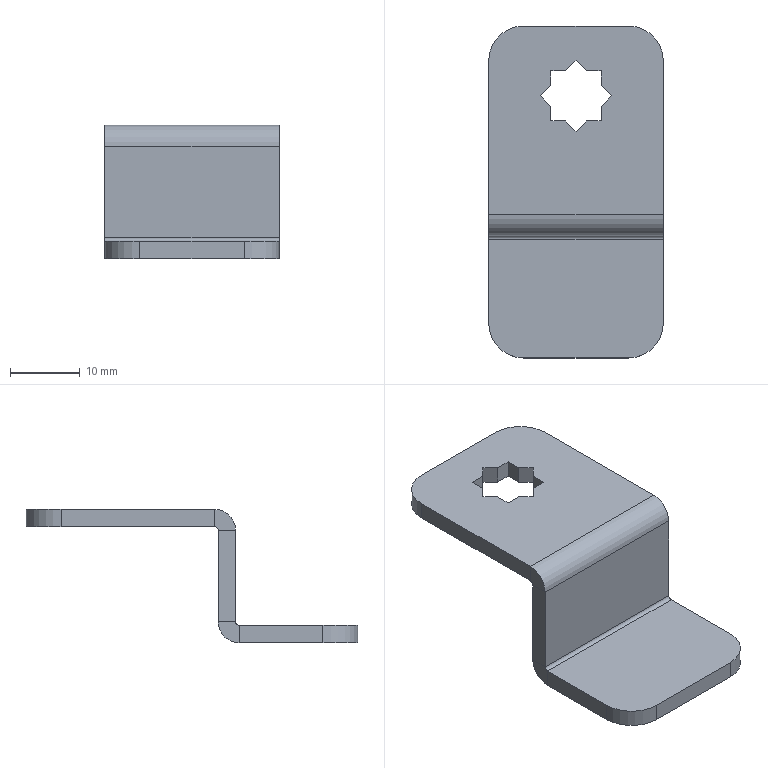Part | SolidWorks | features BaseBody 1 | 1 solid | 42 faces | box 25 x 47.5 x 19.1 mm | volume 3707 mm3 | plane 34 | cylinder 8 | commonest cylinder face diameters 10 x4 1 x2 6 x2
STEP:
#1=CARTESIAN_POINT('',(5.091,5.,0.));
#2=VERTEX_POINT('',#1);
#3=CARTESIAN_POINT('',(3.6,3.509,0.));
#4=VERTEX_POINT('',#3);
#5=CARTESIAN_POINT('',(5.091,5.,0.));
#6=DIRECTION('',(-0.7071,-0.7071,0.));
#7=VECTOR('',#6,1000.);
#8=LINE('',#5,#7);
#9=EDGE_CURVE('',#2,#4,#8,.T.);
#10=ORIENTED_EDGE('',*,*,#9,.F.);
#11=CARTESIAN_POINT('',(5.091,5.,-2.5));
#12=VERTEX_POINT('',#11);
#13=CARTESIAN_POINT('',(5.091,5.,0.));
#14=DIRECTION('',(0.,0.,-1.));
#15=VECTOR('',#14,1000.);
#16=LINE('',#13,#15);
#17=EDGE_CURVE('',#2,#12,#16,.T.);
#18=ORIENTED_EDGE('',*,*,#17,.T.);
#19=CARTESIAN_POINT('',(3.6,3.509,-2.5));
#20=VERTEX_POINT('',#19);
#21=CARTESIAN_POINT('',(5.091,5.,-2.5));
#22=DIRECTION('',(-0.7071,-0.7071,0.));
#23=VECTOR('',#22,1000.);
#24=LINE('',#21,#23);
#25=EDGE_CURVE('',#12,#20,#24,.T.);
#26=ORIENTED_EDGE('',*,*,#25,.T.);
#27=CARTESIAN_POINT('',(3.6,3.509,0.));
#28=DIRECTION('',(0.,0.,-1.));
#29=VECTOR('',#28,1000.);
#30=LINE('',#27,#29);
#31=EDGE_CURVE('',#4,#20,#30,.T.);
#32=ORIENTED_EDGE('',*,*,#31,.F.);
#33=EDGE_LOOP('',(#10,#18,#26,#32));
#34=FACE_OUTER_BOUND('',#33,.T.);
#35=CARTESIAN_POINT('',(5.091,5.,0.));
#36=DIRECTION('',(0.7071,-0.7071,0.));
#37=DIRECTION('',(0.,0.,-1.));
#38=AXIS2_PLACEMENT_3D('',#35,#36,#37);
#39=PLANE('',#38);
#40=ADVANCED_FACE('',(#34),#39,.F.);
#41=CARTESIAN_POINT('',(3.6,6.491,-2.5));
#42=VERTEX_POINT('',#41);
#43=CARTESIAN_POINT('',(0.,10.091,-2.5));
#44=DIRECTION('',(0.7071,-0.7071,0.));
#45=VECTOR('',#44,1000.);
#46=LINE('',#43,#45);
#47=EDGE_CURVE('',#42,#12,#46,.T.);
#48=ORIENTED_EDGE('',*,*,#47,.T.);
#49=ORIENTED_EDGE('',*,*,#17,.F.);
#50=CARTESIAN_POINT('',(3.6,6.491,0.));
#51=VERTEX_POINT('',#50);
#52=CARTESIAN_POINT('',(0.,10.091,0.));
#53=DIRECTION('',(0.7071,-0.7071,0.));
#54=VECTOR('',#53,1000.);
#55=LINE('',#52,#54);
#56=EDGE_CURVE('',#51,#2,#55,.T.);
#57=ORIENTED_EDGE('',*,*,#56,.F.);
#58=CARTESIAN_POINT('',(3.6,6.491,0.));
#59=DIRECTION('',(0.,0.,1.));
#60=VECTOR('',#59,1000.);
#61=LINE('',#58,#60);
#62=EDGE_CURVE('',#42,#51,#61,.T.);
#63=ORIENTED_EDGE('',*,*,#62,.F.);
#64=EDGE_LOOP('',(#48,#49,#57,#63));
#65=FACE_OUTER_BOUND('',#64,.T.);
#66=CARTESIAN_POINT('',(0.,10.091,0.));
#67=DIRECTION('',(0.7071,0.7071,0.));
#68=DIRECTION('',(0.,0.,-1.));
#69=AXIS2_PLACEMENT_3D('',#66,#67,#68);
#70=PLANE('',#69);
#71=ADVANCED_FACE('',(#65),#70,.F.);
#72=CARTESIAN_POINT('',(0.,10.091,0.));
#73=VERTEX_POINT('',#72);
#74=CARTESIAN_POINT('',(1.491,8.6,0.));
#75=VERTEX_POINT('',#74);
#76=CARTESIAN_POINT('',(0.,10.091,0.));
#77=DIRECTION('',(0.7071,-0.7071,0.));
#78=VECTOR('',#77,1000.);
#79=LINE('',#76,#78);
#80=EDGE_CURVE('',#73,#75,#79,.T.);
#81=ORIENTED_EDGE('',*,*,#80,.F.);
#82=CARTESIAN_POINT('',(0.,10.091,-2.5));
#83=VERTEX_POINT('',#82);
#84=CARTESIAN_POINT('',(0.,10.091,0.));
#85=DIRECTION('',(0.,0.,-1.));
#86=VECTOR('',#85,1000.);
#87=LINE('',#84,#86);
#88=EDGE_CURVE('',#73,#83,#87,.T.);
#89=ORIENTED_EDGE('',*,*,#88,.T.);
#90=CARTESIAN_POINT('',(1.491,8.6,-2.5));
#91=VERTEX_POINT('',#90);
#92=CARTESIAN_POINT('',(0.,10.091,-2.5));
#93=DIRECTION('',(0.7071,-0.7071,0.));
#94=VECTOR('',#93,1000.);
#95=LINE('',#92,#94);
#96=EDGE_CURVE('',#83,#91,#95,.T.);
#97=ORIENTED_EDGE('',*,*,#96,.T.);
#98=CARTESIAN_POINT('',(1.491,8.6,0.));
#99=DIRECTION('',(0.,0.,-1.));
#100=VECTOR('',#99,1000.);
#101=LINE('',#98,#100);
#102=EDGE_CURVE('',#75,#91,#101,.T.);
#103=ORIENTED_EDGE('',*,*,#102,.F.);
#104=EDGE_LOOP('',(#81,#89,#97,#103));
#105=FACE_OUTER_BOUND('',#104,.T.);
#106=CARTESIAN_POINT('',(0.,10.091,0.));
#107=DIRECTION('',(0.7071,0.7071,0.));
#108=DIRECTION('',(0.,0.,-1.));
#109=AXIS2_PLACEMENT_3D('',#106,#107,#108);
#110=PLANE('',#109);
#111=ADVANCED_FACE('',(#105),#110,.F.);
#112=CARTESIAN_POINT('',(-1.491,8.6,-2.5));
#113=VERTEX_POINT('',#112);
#114=CARTESIAN_POINT('',(0.,10.091,-2.5));
#115=DIRECTION('',(0.7071,0.7071,0.));
#116=VECTOR('',#115,1000.);
#117=LINE('',#114,#116);
#118=EDGE_CURVE('',#113,#83,#117,.T.);
#119=ORIENTED_EDGE('',*,*,#118,.T.);
#120=ORIENTED_EDGE('',*,*,#88,.F.);
#121=CARTESIAN_POINT('',(-1.491,8.6,0.));
#122=VERTEX_POINT('',#121);
#123=CARTESIAN_POINT('',(0.,10.091,0.));
#124=DIRECTION('',(0.7071,0.7071,0.));
#125=VECTOR('',#124,1000.);
#126=LINE('',#123,#125);
#127=EDGE_CURVE('',#122,#73,#126,.T.);
#128=ORIENTED_EDGE('',*,*,#127,.F.);
#129=CARTESIAN_POINT('',(-1.491,8.6,0.));
#130=DIRECTION('',(0.,0.,1.));
#131=VECTOR('',#130,1000.);
#132=LINE('',#129,#131);
#133=EDGE_CURVE('',#113,#122,#132,.T.);
#134=ORIENTED_EDGE('',*,*,#133,.F.);
#135=EDGE_LOOP('',(#119,#120,#128,#134));
#136=FACE_OUTER_BOUND('',#135,.T.);
#137=CARTESIAN_POINT('',(0.,10.091,0.));
#138=DIRECTION('',(-0.7071,0.7071,0.));
#139=DIRECTION('',(0.,0.,1.));
#140=AXIS2_PLACEMENT_3D('',#137,#138,#139);
#141=PLANE('',#140);
#142=ADVANCED_FACE('',(#136),#141,.F.);
#143=CARTESIAN_POINT('',(-5.091,5.,0.));
#144=VERTEX_POINT('',#143);
#145=CARTESIAN_POINT('',(-3.6,6.491,0.));
#146=VERTEX_POINT('',#145);
#147=CARTESIAN_POINT('',(0.,10.091,0.));
#148=DIRECTION('',(0.7071,0.7071,0.));
#149=VECTOR('',#148,1000.);
#150=LINE('',#147,#149);
#151=EDGE_CURVE('',#144,#146,#150,.T.);
#152=ORIENTED_EDGE('',*,*,#151,.F.);
#153=CARTESIAN_POINT('',(-5.091,5.,-2.5));
#154=VERTEX_POINT('',#153);
#155=CARTESIAN_POINT('',(-5.091,5.,0.));
#156=DIRECTION('',(0.,0.,-1.));
#157=VECTOR('',#156,1000.);
#158=LINE('',#155,#157);
#159=EDGE_CURVE('',#144,#154,#158,.T.);
#160=ORIENTED_EDGE('',*,*,#159,.T.);
#161=CARTESIAN_POINT('',(-3.6,6.491,-2.5));
#162=VERTEX_POINT('',#161);
#163=CARTESIAN_POINT('',(0.,10.091,-2.5));
#164=DIRECTION('',(0.7071,0.7071,0.));
#165=VECTOR('',#164,1000.);
#166=LINE('',#163,#165);
#167=EDGE_CURVE('',#154,#162,#166,.T.);
#168=ORIENTED_EDGE('',*,*,#167,.T.);
#169=CARTESIAN_POINT('',(-3.6,6.491,0.));
#170=DIRECTION('',(0.,0.,-1.));
#171=VECTOR('',#170,1000.);
#172=LINE('',#169,#171);
#173=EDGE_CURVE('',#146,#162,#172,.T.);
#174=ORIENTED_EDGE('',*,*,#173,.F.);
#175=EDGE_LOOP('',(#152,#160,#168,#174));
#176=FACE_OUTER_BOUND('',#175,.T.);
#177=CARTESIAN_POINT('',(0.,10.091,0.));
#178=DIRECTION('',(-0.7071,0.7071,0.));
#179=DIRECTION('',(0.,0.,1.));
#180=AXIS2_PLACEMENT_3D('',#177,#178,#179);
#181=PLANE('',#180);
#182=ADVANCED_FACE('',(#176),#181,.F.);
#183=CARTESIAN_POINT('',(-3.6,3.509,-2.5));
#184=VERTEX_POINT('',#183);
#185=CARTESIAN_POINT('',(-5.091,5.,-2.5));
#186=DIRECTION('',(-0.7071,0.7071,0.));
#187=VECTOR('',#186,1000.);
#188=LINE('',#185,#187);
#189=EDGE_CURVE('',#184,#154,#188,.T.);
#190=ORIENTED_EDGE('',*,*,#189,.T.);
#191=ORIENTED_EDGE('',*,*,#159,.F.);
#192=CARTESIAN_POINT('',(-3.6,3.509,0.));
#193=VERTEX_POINT('',#192);
#194=CARTESIAN_POINT('',(-5.091,5.,0.));
#195=DIRECTION('',(-0.7071,0.7071,0.));
#196=VECTOR('',#195,1000.);
#197=LINE('',#194,#196);
#198=EDGE_CURVE('',#193,#144,#197,.T.);
#199=ORIENTED_EDGE('',*,*,#198,.F.);
#200=CARTESIAN_POINT('',(-3.6,3.509,0.));
#201=DIRECTION('',(0.,0.,1.));
#202=VECTOR('',#201,1000.);
#203=LINE('',#200,#202);
#204=EDGE_CURVE('',#184,#193,#203,.T.);
#205=ORIENTED_EDGE('',*,*,#204,.F.);
#206=EDGE_LOOP('',(#190,#191,#199,#205));
#207=FACE_OUTER_BOUND('',#206,.T.);
#208=CARTESIAN_POINT('',(-5.091,5.,0.));
#209=DIRECTION('',(-0.7071,-0.7071,0.));
#210=DIRECTION('',(-0.7071,0.7071,0.));
#211=AXIS2_PLACEMENT_3D('',#208,#209,#210);
#212=PLANE('',#211);
#213=ADVANCED_FACE('',(#207),#212,.F.);
#214=CARTESIAN_POINT('',(1.491,1.4,-2.5));
#215=VERTEX_POINT('',#214);
#216=CARTESIAN_POINT('',(0.,-0.09117,-2.5));
#217=VERTEX_POINT('',#216);
#218=CARTESIAN_POINT('',(5.091,5.,-2.5));
#219=DIRECTION('',(-0.7071,-0.7071,0.));
#220=VECTOR('',#219,1000.);
#221=LINE('',#218,#220);
#222=EDGE_CURVE('',#215,#217,#221,.T.);
#223=ORIENTED_EDGE('',*,*,#222,.T.);
#224=CARTESIAN_POINT('',(0.,-0.09117,0.));
#225=VERTEX_POINT('',#224);
#226=CARTESIAN_POINT('',(0.,-0.09117,0.));
#227=DIRECTION('',(0.,0.,-1.));
#228=VECTOR('',#227,1000.);
#229=LINE('',#226,#228);
#230=EDGE_CURVE('',#225,#217,#229,.T.);
#231=ORIENTED_EDGE('',*,*,#230,.F.);
#232=CARTESIAN_POINT('',(1.491,1.4,0.));
#233=VERTEX_POINT('',#232);
#234=CARTESIAN_POINT('',(5.091,5.,0.));
#235=DIRECTION('',(-0.7071,-0.7071,0.));
#236=VECTOR('',#235,1000.);
#237=LINE('',#234,#236);
#238=EDGE_CURVE('',#233,#225,#237,.T.);
#239=ORIENTED_EDGE('',*,*,#238,.F.);
#240=CARTESIAN_POINT('',(1.491,1.4,0.));
#241=DIRECTION('',(0.,0.,1.));
#242=VECTOR('',#241,1000.);
#243=LINE('',#240,#242);
#244=EDGE_CURVE('',#215,#233,#243,.T.);
#245=ORIENTED_EDGE('',*,*,#244,.F.);
#246=EDGE_LOOP('',(#223,#231,#239,#245));
#247=FACE_OUTER_BOUND('',#246,.T.);
#248=CARTESIAN_POINT('',(5.091,5.,0.));
#249=DIRECTION('',(0.7071,-0.7071,0.));
#250=DIRECTION('',(0.,0.,-1.));
#251=AXIS2_PLACEMENT_3D('',#248,#249,#250);
#252=PLANE('',#251);
#253=ADVANCED_FACE('',(#247),#252,.F.);
#254=CARTESIAN_POINT('',(-1.491,1.4,0.));
#255=VERTEX_POINT('',#254);
#256=CARTESIAN_POINT('',(-5.091,5.,0.));
#257=DIRECTION('',(-0.7071,0.7071,0.));
#258=VECTOR('',#257,1000.);
#259=LINE('',#256,#258);
#260=EDGE_CURVE('',#225,#255,#259,.T.);
#261=ORIENTED_EDGE('',*,*,#260,.F.);
#262=ORIENTED_EDGE('',*,*,#230,.T.);
#263=CARTESIAN_POINT('',(-1.491,1.4,-2.5));
#264=VERTEX_POINT('',#263);
#265=CARTESIAN_POINT('',(-5.091,5.,-2.5));
#266=DIRECTION('',(-0.7071,0.7071,0.));
#267=VECTOR('',#266,1000.);
#268=LINE('',#265,#267);
#269=EDGE_CURVE('',#217,#264,#268,.T.);
#270=ORIENTED_EDGE('',*,*,#269,.T.);
#271=CARTESIAN_POINT('',(-1.491,1.4,0.));
#272=DIRECTION('',(0.,0.,-1.));
#273=VECTOR('',#272,1000.);
#274=LINE('',#271,#273);
#275=EDGE_CURVE('',#255,#264,#274,.T.);
#276=ORIENTED_EDGE('',*,*,#275,.F.);
#277=EDGE_LOOP('',(#261,#262,#270,#276));
#278=FACE_OUTER_BOUND('',#277,.T.);
#279=CARTESIAN_POINT('',(-5.091,5.,0.));
#280=DIRECTION('',(-0.7071,-0.7071,0.));
#281=DIRECTION('',(-0.7071,0.7071,0.));
#282=AXIS2_PLACEMENT_3D('',#279,#280,#281);
#283=PLANE('',#282);
#284=ADVANCED_FACE('',(#278),#283,.F.);
#285=CARTESIAN_POINT('',(-3.6,1.4,0.));
#286=VERTEX_POINT('',#285);
#287=CARTESIAN_POINT('',(-3.6,1.4,0.));
#288=DIRECTION('',(-1.,0.,0.));
#289=VECTOR('',#288,1000.);
#290=LINE('',#287,#289);
#291=EDGE_CURVE('',#255,#286,#290,.T.);
#292=ORIENTED_EDGE('',*,*,#291,.F.);
#293=ORIENTED_EDGE('',*,*,#275,.T.);
#294=CARTESIAN_POINT('',(-3.6,1.4,-2.5));
#295=VERTEX_POINT('',#294);
#296=CARTESIAN_POINT('',(-3.6,1.4,-2.5));
#297=DIRECTION('',(-1.,0.,0.));
#298=VECTOR('',#297,1000.);
#299=LINE('',#296,#298);
#300=EDGE_CURVE('',#264,#295,#299,.T.);
#301=ORIENTED_EDGE('',*,*,#300,.T.);
#302=CARTESIAN_POINT('',(-3.6,1.4,0.));
#303=DIRECTION('',(0.,0.,-1.));
#304=VECTOR('',#303,1000.);
#305=LINE('',#302,#304);
#306=EDGE_CURVE('',#286,#295,#305,.T.);
#307=ORIENTED_EDGE('',*,*,#306,.F.);
#308=EDGE_LOOP('',(#292,#293,#301,#307));
#309=FACE_OUTER_BOUND('',#308,.T.);
#310=CARTESIAN_POINT('',(-3.6,1.4,0.));
#311=DIRECTION('',(0.,-1.,0.));
#312=DIRECTION('',(-1.,0.,0.));
#313=AXIS2_PLACEMENT_3D('',#310,#311,#312);
#314=PLANE('',#313);
#315=ADVANCED_FACE('',(#309),#314,.F.);
#316=CARTESIAN_POINT('',(-3.6,8.6,-2.5));
#317=DIRECTION('',(0.,1.,0.));
#318=VECTOR('',#317,1000.);
#319=LINE('',#316,#318);
#320=EDGE_CURVE('',#295,#184,#319,.T.);
#321=ORIENTED_EDGE('',*,*,#320,.T.);
#322=ORIENTED_EDGE('',*,*,#204,.T.);
#323=CARTESIAN_POINT('',(-3.6,8.6,0.));
#324=DIRECTION('',(0.,1.,0.));
#325=VECTOR('',#324,1000.);
#326=LINE('',#323,#325);
#327=EDGE_CURVE('',#286,#193,#326,.T.);
#328=ORIENTED_EDGE('',*,*,#327,.F.);
#329=ORIENTED_EDGE('',*,*,#306,.T.);
#330=EDGE_LOOP('',(#321,#322,#328,#329));
#331=FACE_OUTER_BOUND('',#330,.T.);
#332=CARTESIAN_POINT('',(-3.6,8.6,0.));
#333=DIRECTION('',(-1.,0.,0.));
#334=DIRECTION('',(0.,0.,1.));
#335=AXIS2_PLACEMENT_3D('',#332,#333,#334);
#336=PLANE('',#335);
#337=ADVANCED_FACE('',(#331),#336,.F.);
#338=CARTESIAN_POINT('',(-3.6,8.6,-2.5));
#339=VERTEX_POINT('',#338);
#340=CARTESIAN_POINT('',(-3.6,8.6,-2.5));
#341=DIRECTION('',(1.,0.,0.));
#342=VECTOR('',#341,1000.);
#343=LINE('',#340,#342);
#344=EDGE_CURVE('',#339,#113,#343,.T.);
#345=ORIENTED_EDGE('',*,*,#344,.T.);
#346=ORIENTED_EDGE('',*,*,#133,.T.);
#347=CARTESIAN_POINT('',(-3.6,8.6,0.));
#348=VERTEX_POINT('',#347);
#349=CARTESIAN_POINT('',(-3.6,8.6,0.));
#350=DIRECTION('',(1.,0.,0.));
#351=VECTOR('',#350,1000.);
#352=LINE('',#349,#351);
#353=EDGE_CURVE('',#348,#122,#352,.T.);
#354=ORIENTED_EDGE('',*,*,#353,.F.);
#355=CARTESIAN_POINT('',(-3.6,8.6,0.));
#356=DIRECTION('',(0.,0.,-1.));
#357=VECTOR('',#356,1000.);
#358=LINE('',#355,#357);
#359=EDGE_CURVE('',#348,#339,#358,.T.);
#360=ORIENTED_EDGE('',*,*,#359,.T.);
#361=EDGE_LOOP('',(#345,#346,#354,#360));
#362=FACE_OUTER_BOUND('',#361,.T.);
#363=CARTESIAN_POINT('',(-3.6,8.6,0.));
#364=DIRECTION('',(0.,1.,0.));
#365=DIRECTION('',(0.,0.,-1.));
#366=AXIS2_PLACEMENT_3D('',#363,#364,#365);
#367=PLANE('',#366);
#368=ADVANCED_FACE('',(#362),#367,.F.);
#369=CARTESIAN_POINT('',(3.6,8.6,-2.5));
#370=VERTEX_POINT('',#369);
#371=CARTESIAN_POINT('',(3.6,8.6,-2.5));
#372=DIRECTION('',(0.,-1.,0.));
#373=VECTOR('',#372,1000.);
#374=LINE('',#371,#373);
#375=EDGE_CURVE('',#370,#42,#374,.T.);
#376=ORIENTED_EDGE('',*,*,#375,.T.);
#377=ORIENTED_EDGE('',*,*,#62,.T.);
#378=CARTESIAN_POINT('',(3.6,8.6,0.));
#379=VERTEX_POINT('',#378);
#380=CARTESIAN_POINT('',(3.6,8.6,0.));
#381=DIRECTION('',(0.,-1.,0.));
#382=VECTOR('',#381,1000.);
#383=LINE('',#380,#382);
#384=EDGE_CURVE('',#379,#51,#383,.T.);
#385=ORIENTED_EDGE('',*,*,#384,.F.);
#386=CARTESIAN_POINT('',(3.6,8.6,0.));
#387=DIRECTION('',(0.,0.,-1.));
#388=VECTOR('',#387,1000.);
#389=LINE('',#386,#388);
#390=EDGE_CURVE('',#379,#370,#389,.T.);
#391=ORIENTED_EDGE('',*,*,#390,.T.);
#392=EDGE_LOOP('',(#376,#377,#385,#391));
#393=FACE_OUTER_BOUND('',#392,.T.);
#394=CARTESIAN_POINT('',(3.6,8.6,0.));
#395=DIRECTION('',(1.,0.,0.));
#396=DIRECTION('',(0.,1.,0.));
#397=AXIS2_PLACEMENT_3D('',#394,#395,#396);
#398=PLANE('',#397);
#399=ADVANCED_FACE('',(#393),#398,.F.);
#400=CARTESIAN_POINT('',(-7.5,-32.5,-19.1));
#401=VERTEX_POINT('',#400);
#402=CARTESIAN_POINT('',(-12.5,-27.5,-19.1));
#403=VERTEX_POINT('',#402);
#404=CARTESIAN_POINT('',(-7.5,-27.5,-19.1));
#405=DIRECTION('',(0.,0.,-1.));
#406=DIRECTION('',(1.,0.,0.));
#407=AXIS2_PLACEMENT_3D('',#404,#405,#406);
#408=CIRCLE('',#407,5.);
#409=EDGE_CURVE('',#401,#403,#408,.T.);
#410=ORIENTED_EDGE('',*,*,#409,.F.);
#411=CARTESIAN_POINT('',(-7.5,-32.5,-16.6));
#412=VERTEX_POINT('',#411);
#413=CARTESIAN_POINT('',(-7.5,-32.5,-19.1));
#414=DIRECTION('',(0.,0.,-1.));
#415=VECTOR('',#414,1000.);
#416=LINE('',#413,#415);
#417=EDGE_CURVE('',#412,#401,#416,.T.);
#418=ORIENTED_EDGE('',*,*,#417,.F.);
#419=CARTESIAN_POINT('',(-12.5,-27.5,-16.6));
#420=VERTEX_POINT('',#419);
#421=CARTESIAN_POINT('',(-7.5,-27.5,-16.6));
#422=DIRECTION('',(0.,0.,1.));
#423=DIRECTION('',(1.,0.,0.));
#424=AXIS2_PLACEMENT_3D('',#421,#422,#423);
#425=CIRCLE('',#424,5.);
#426=EDGE_CURVE('',#420,#412,#425,.T.);
#427=ORIENTED_EDGE('',*,*,#426,.F.);
#428=CARTESIAN_POINT('',(-12.5,-27.5,-19.1));
#429=DIRECTION('',(0.,0.,1.));
#430=VECTOR('',#429,1000.);
#431=LINE('',#428,#430);
#432=EDGE_CURVE('',#403,#420,#431,.T.);
#433=ORIENTED_EDGE('',*,*,#432,.F.);
#434=EDGE_LOOP('',(#410,#418,#427,#433));
#435=FACE_OUTER_BOUND('',#434,.T.);
#436=CARTESIAN_POINT('',(-7.5,-27.5,-19.1));
#437=DIRECTION('',(0.,0.,1.));
#438=DIRECTION('',(0.,-1.,0.));
#439=AXIS2_PLACEMENT_3D('',#436,#437,#438);
#440=CYLINDRICAL_SURFACE('',#439,5.);
#441=ADVANCED_FACE('',(#435),#440,.T.);
#442=CARTESIAN_POINT('',(-12.5,10.,-2.5));
#443=VERTEX_POINT('',#442);
#444=CARTESIAN_POINT('',(-7.5,15.,-2.5));
#445=VERTEX_POINT('',#444);
#446=CARTESIAN_POINT('',(-7.5,10.,-2.5));
#447=DIRECTION('',(0.,0.,-1.));
#448=DIRECTION('',(-1.,0.,0.));
#449=AXIS2_PLACEMENT_3D('',#446,#447,#448);
#450=CIRCLE('',#449,5.);
#451=EDGE_CURVE('',#443,#445,#450,.T.);
#452=ORIENTED_EDGE('',*,*,#451,.F.);
#453=CARTESIAN_POINT('',(-12.5,10.,0.));
#454=VERTEX_POINT('',#453);
#455=CARTESIAN_POINT('',(-12.5,10.,-2.5));
#456=DIRECTION('',(0.,0.,-1.));
#457=VECTOR('',#456,1000.);
#458=LINE('',#455,#457);
#459=EDGE_CURVE('',#454,#443,#458,.T.);
#460=ORIENTED_EDGE('',*,*,#459,.F.);
#461=CARTESIAN_POINT('',(-7.5,15.,0.));
#462=VERTEX_POINT('',#461);
#463=CARTESIAN_POINT('',(-7.5,10.,0.));
#464=DIRECTION('',(0.,0.,1.));
#465=DIRECTION('',(-1.,0.,0.));
#466=AXIS2_PLACEMENT_3D('',#463,#464,#465);
#467=CIRCLE('',#466,5.);
#468=EDGE_CURVE('',#462,#454,#467,.T.);
#469=ORIENTED_EDGE('',*,*,#468,.F.);
#470=CARTESIAN_POINT('',(-7.5,15.,-2.5));
#471=DIRECTION('',(0.,0.,1.));
#472=VECTOR('',#471,1000.);
#473=LINE('',#470,#472);
#474=EDGE_CURVE('',#445,#462,#473,.T.);
#475=ORIENTED_EDGE('',*,*,#474,.F.);
#476=EDGE_LOOP('',(#452,#460,#469,#475));
#477=FACE_OUTER_BOUND('',#476,.T.);
#478=CARTESIAN_POINT('',(-7.5,10.,-2.5));
#479=DIRECTION('',(0.,0.,1.));
#480=DIRECTION('',(1.,0.,0.));
#481=AXIS2_PLACEMENT_3D('',#478,#479,#480);
#482=CYLINDRICAL_SURFACE('',#481,5.);
#483=ADVANCED_FACE('',(#477),#482,.T.);
#484=CARTESIAN_POINT('',(7.5,15.,-2.5));
#485=VERTEX_POINT('',#484);
#486=CARTESIAN_POINT('',(12.5,10.,-2.5));
#487=VERTEX_POINT('',#486);
#488=CARTESIAN_POINT('',(7.5,10.,-2.5));
#489=DIRECTION('',(0.,0.,-1.));
#490=DIRECTION('',(-1.,0.,0.));
#491=AXIS2_PLACEMENT_3D('',#488,#489,#490);
#492=CIRCLE('',#491,5.);
#493=EDGE_CURVE('',#485,#487,#492,.T.);
#494=ORIENTED_EDGE('',*,*,#493,.F.);
#495=CARTESIAN_POINT('',(7.5,15.,0.));
#496=VERTEX_POINT('',#495);
#497=CARTESIAN_POINT('',(7.5,15.,-2.5));
#498=DIRECTION('',(0.,0.,-1.));
#499=VECTOR('',#498,1000.);
#500=LINE('',#497,#499);
#501=EDGE_CURVE('',#496,#485,#500,.T.);
#502=ORIENTED_EDGE('',*,*,#501,.F.);
#503=CARTESIAN_POINT('',(12.5,10.,0.));
#504=VERTEX_POINT('',#503);
#505=CARTESIAN_POINT('',(7.5,10.,0.));
#506=DIRECTION('',(0.,0.,1.));
#507=DIRECTION('',(-1.,0.,0.));
#508=AXIS2_PLACEMENT_3D('',#505,#506,#507);
#509=CIRCLE('',#508,5.);
#510=EDGE_CURVE('',#504,#496,#509,.T.);
#511=ORIENTED_EDGE('',*,*,#510,.F.);
#512=CARTESIAN_POINT('',(12.5,10.,-2.5));
#513=DIRECTION('',(0.,0.,1.));
#514=VECTOR('',#513,1000.);
#515=LINE('',#512,#514);
#516=EDGE_CURVE('',#487,#504,#515,.T.);
#517=ORIENTED_EDGE('',*,*,#516,.F.);
#518=EDGE_LOOP('',(#494,#502,#511,#517));
#519=FACE_OUTER_BOUND('',#518,.T.);
#520=CARTESIAN_POINT('',(7.5,10.,-2.5));
#521=DIRECTION('',(0.,0.,1.));
#522=DIRECTION('',(1.,0.,0.));
#523=AXIS2_PLACEMENT_3D('',#520,#521,#522);
#524=CYLINDRICAL_SURFACE('',#523,5.);
#525=ADVANCED_FACE('',(#519),#524,.T.);
#526=CARTESIAN_POINT('',(12.5,-27.5,-19.1));
#527=VERTEX_POINT('',#526);
#528=CARTESIAN_POINT('',(7.5,-32.5,-19.1));
#529=VERTEX_POINT('',#528);
#530=CARTESIAN_POINT('',(7.5,-27.5,-19.1));
#531=DIRECTION('',(0.,0.,-1.));
#532=DIRECTION('',(1.,0.,0.));
#533=AXIS2_PLACEMENT_3D('',#530,#531,#532);
#534=CIRCLE('',#533,5.);
#535=EDGE_CURVE('',#527,#529,#534,.T.);
#536=ORIENTED_EDGE('',*,*,#535,.F.);
#537=CARTESIAN_POINT('',(12.5,-27.5,-16.6));
#538=VERTEX_POINT('',#537);
#539=CARTESIAN_POINT('',(12.5,-27.5,-19.1));
#540=DIRECTION('',(0.,0.,-1.));
#541=VECTOR('',#540,1000.);
#542=LINE('',#539,#541);
#543=EDGE_CURVE('',#538,#527,#542,.T.);
#544=ORIENTED_EDGE('',*,*,#543,.F.);
#545=CARTESIAN_POINT('',(7.5,-32.5,-16.6));
#546=VERTEX_POINT('',#545);
#547=CARTESIAN_POINT('',(7.5,-27.5,-16.6));
#548=DIRECTION('',(0.,0.,1.));
#549=DIRECTION('',(1.,0.,0.));
#550=AXIS2_PLACEMENT_3D('',#547,#548,#549);
#551=CIRCLE('',#550,5.);
#552=EDGE_CURVE('',#546,#538,#551,.T.);
#553=ORIENTED_EDGE('',*,*,#552,.F.);
#554=CARTESIAN_POINT('',(7.5,-32.5,-19.1));
#555=DIRECTION('',(0.,0.,1.));
#556=VECTOR('',#555,1000.);
#557=LINE('',#554,#556);
#558=EDGE_CURVE('',#529,#546,#557,.T.);
#559=ORIENTED_EDGE('',*,*,#558,.F.);
#560=EDGE_LOOP('',(#536,#544,#553,#559));
#561=FACE_OUTER_BOUND('',#560,.T.);
#562=CARTESIAN_POINT('',(7.5,-27.5,-19.1));
#563=DIRECTION('',(0.,0.,1.));
#564=DIRECTION('',(0.,-1.,0.));
#565=AXIS2_PLACEMENT_3D('',#562,#563,#564);
#566=CYLINDRICAL_SURFACE('',#565,5.);
#567=ADVANCED_FACE('',(#561),#566,.T.);
#568=CARTESIAN_POINT('',(0.,-32.5,-19.1));
#569=DIRECTION('',(-1.,0.,0.));
#570=VECTOR('',#569,1000.);
#571=LINE('',#568,#570);
#572=EDGE_CURVE('',#529,#401,#571,.T.);
#573=ORIENTED_EDGE('',*,*,#572,.F.);
#574=ORIENTED_EDGE('',*,*,#558,.T.);
#575=CARTESIAN_POINT('',(-12.5,-32.5,-16.6));
#576=DIRECTION('',(-1.,0.,0.));
#577=VECTOR('',#576,1000.);
#578=LINE('',#575,#577);
#579=EDGE_CURVE('',#546,#412,#578,.T.);
#580=ORIENTED_EDGE('',*,*,#579,.T.);
#581=ORIENTED_EDGE('',*,*,#417,.T.);
#582=EDGE_LOOP('',(#573,#574,#580,#581));
#583=FACE_OUTER_BOUND('',#582,.T.);
#584=CARTESIAN_POINT('',(-12.5,-32.5,-19.1));
#585=DIRECTION('',(0.,1.,0.));
#586=DIRECTION('',(0.,0.,-1.));
#587=AXIS2_PLACEMENT_3D('',#584,#585,#586);
#588=PLANE('',#587);
#589=ADVANCED_FACE('',(#583),#588,.F.);
#590=ORIENTED_EDGE('',*,*,#579,.F.);
#591=ORIENTED_EDGE('',*,*,#552,.T.);
#592=CARTESIAN_POINT('',(12.5,-15.5,-16.6));
#593=VERTEX_POINT('',#592);
#594=CARTESIAN_POINT('',(12.5,-32.5,-16.6));
#595=DIRECTION('',(0.,-1.,0.));
#596=VECTOR('',#595,1000.);
#597=LINE('',#594,#596);
#598=EDGE_CURVE('',#593,#538,#597,.T.);
#599=ORIENTED_EDGE('',*,*,#598,.F.);
#600=CARTESIAN_POINT('',(-12.5,-15.5,-16.6));
#601=VERTEX_POINT('',#600);
#602=CARTESIAN_POINT('',(-12.5,-15.5,-16.6));
#603=DIRECTION('',(1.,0.,0.));
#604=VECTOR('',#603,1000.);
#605=LINE('',#602,#604);
#606=EDGE_CURVE('',#601,#593,#605,.T.);
#607=ORIENTED_EDGE('',*,*,#606,.F.);
#608=CARTESIAN_POINT('',(-12.5,-15.,-16.6));
#609=DIRECTION('',(0.,1.,0.));
#610=VECTOR('',#609,1000.);
#611=LINE('',#608,#610);
#612=EDGE_CURVE('',#420,#601,#611,.T.);
#613=ORIENTED_EDGE('',*,*,#612,.F.);
#614=ORIENTED_EDGE('',*,*,#426,.T.);
#615=EDGE_LOOP('',(#590,#591,#599,#607,#613,#614));
#616=FACE_OUTER_BOUND('',#615,.T.);
#617=CARTESIAN_POINT('',(0.,0.,-16.6));
#618=DIRECTION('',(0.,0.,1.));
#619=DIRECTION('',(1.,0.,0.));
#620=AXIS2_PLACEMENT_3D('',#617,#618,#619);
#621=PLANE('',#620);
#622=ADVANCED_FACE('',(#616),#621,.T.);
#623=CARTESIAN_POINT('',(12.5,-15.5,-19.1));
#624=VERTEX_POINT('',#623);
#625=CARTESIAN_POINT('',(12.5,0.,-19.1));
#626=DIRECTION('',(0.,-1.,0.));
#627=VECTOR('',#626,1000.);
#628=LINE('',#625,#627);
#629=EDGE_CURVE('',#624,#527,#628,.T.);
#630=ORIENTED_EDGE('',*,*,#629,.T.);
#631=ORIENTED_EDGE('',*,*,#535,.T.);
#632=ORIENTED_EDGE('',*,*,#572,.T.);
#633=ORIENTED_EDGE('',*,*,#409,.T.);
#634=CARTESIAN_POINT('',(-12.5,-15.5,-19.1));
#635=VERTEX_POINT('',#634);
#636=CARTESIAN_POINT('',(-12.5,0.,-19.1));
#637=DIRECTION('',(0.,1.,0.));
#638=VECTOR('',#637,1000.);
#639=LINE('',#636,#638);
#640=EDGE_CURVE('',#403,#635,#639,.T.);
#641=ORIENTED_EDGE('',*,*,#640,.T.);
#642=CARTESIAN_POINT('',(-12.5,-15.5,-19.1));
#643=DIRECTION('',(-1.,0.,0.));
#644=VECTOR('',#643,1000.);
#645=LINE('',#642,#644);
#646=EDGE_CURVE('',#624,#635,#645,.T.);
#647=ORIENTED_EDGE('',*,*,#646,.F.);
#648=EDGE_LOOP('',(#630,#631,#632,#633,#641,#647));
#649=FACE_OUTER_BOUND('',#648,.T.);
#650=CARTESIAN_POINT('',(0.,0.,-19.1));
#651=DIRECTION('',(0.,0.,1.));
#652=DIRECTION('',(1.,0.,0.));
#653=AXIS2_PLACEMENT_3D('',#650,#651,#652);
#654=PLANE('',#653);
#655=ADVANCED_FACE('',(#649),#654,.F.);
#656=ORIENTED_EDGE('',*,*,#640,.F.);
#657=ORIENTED_EDGE('',*,*,#432,.T.);
#658=ORIENTED_EDGE('',*,*,#612,.T.);
#659=CARTESIAN_POINT('',(-12.5,-15.5,-19.1));
#660=DIRECTION('',(0.,0.,-1.));
#661=VECTOR('',#660,1000.);
#662=LINE('',#659,#661);
#663=EDGE_CURVE('',#601,#635,#662,.T.);
#664=ORIENTED_EDGE('',*,*,#663,.T.);
#665=EDGE_LOOP('',(#656,#657,#658,#664));
#666=FACE_OUTER_BOUND('',#665,.T.);
#667=CARTESIAN_POINT('',(-12.5,-15.,-19.1));
#668=DIRECTION('',(1.,0.,0.));
#669=DIRECTION('',(0.,1.,0.));
#670=AXIS2_PLACEMENT_3D('',#667,#668,#669);
#671=PLANE('',#670);
#672=ADVANCED_FACE('',(#666),#671,.F.);
#673=ORIENTED_EDGE('',*,*,#598,.T.);
#674=ORIENTED_EDGE('',*,*,#543,.T.);
#675=ORIENTED_EDGE('',*,*,#629,.F.);
#676=CARTESIAN_POINT('',(12.5,-15.5,-16.6));
#677=DIRECTION('',(0.,0.,-1.));
#678=VECTOR('',#677,1000.);
#679=LINE('',#676,#678);
#680=EDGE_CURVE('',#593,#624,#679,.T.);
#681=ORIENTED_EDGE('',*,*,#680,.F.);
#682=EDGE_LOOP('',(#673,#674,#675,#681));
#683=FACE_OUTER_BOUND('',#682,.T.);
#684=CARTESIAN_POINT('',(12.5,-32.5,-19.1));
#685=DIRECTION('',(-1.,0.,0.));
#686=DIRECTION('',(0.,0.,1.));
#687=AXIS2_PLACEMENT_3D('',#684,#685,#686);
#688=PLANE('',#687);
#689=ADVANCED_FACE('',(#683),#688,.F.);
#690=CARTESIAN_POINT('',(12.5,-15.,-16.1));
#691=VERTEX_POINT('',#690);
#692=CARTESIAN_POINT('',(-12.5,-15.,-16.1));
#693=VERTEX_POINT('',#692);
#694=CARTESIAN_POINT('',(12.5,-15.,-16.1));
#695=DIRECTION('',(-1.,0.,0.));
#696=VECTOR('',#695,1000.);
#697=LINE('',#694,#696);
#698=EDGE_CURVE('',#691,#693,#697,.T.);
#699=ORIENTED_EDGE('',*,*,#698,.T.);
#700=CARTESIAN_POINT('',(-12.5,-15.5,-16.1));
#701=DIRECTION('',(-1.,0.,0.));
#702=DIRECTION('',(0.,0.,-1.));
#703=AXIS2_PLACEMENT_3D('',#700,#701,#702);
#704=CIRCLE('',#703,0.5);
#705=EDGE_CURVE('',#693,#601,#704,.T.);
#706=ORIENTED_EDGE('',*,*,#705,.T.);
#707=ORIENTED_EDGE('',*,*,#606,.T.);
#708=CARTESIAN_POINT('',(12.5,-15.5,-16.1));
#709=DIRECTION('',(1.,0.,0.));
#710=DIRECTION('',(0.,0.,-1.));
#711=AXIS2_PLACEMENT_3D('',#708,#709,#710);
#712=CIRCLE('',#711,0.5);
#713=EDGE_CURVE('',#593,#691,#712,.T.);
#714=ORIENTED_EDGE('',*,*,#713,.T.);
#715=EDGE_LOOP('',(#699,#706,#707,#714));
#716=FACE_OUTER_BOUND('',#715,.T.);
#717=CARTESIAN_POINT('',(12.5,-15.5,-16.1));
#718=DIRECTION('',(1.,0.,0.));
#719=DIRECTION('',(0.,0.,-1.));
#720=AXIS2_PLACEMENT_3D('',#717,#718,#719);
#721=CYLINDRICAL_SURFACE('',#720,0.5);
#722=ADVANCED_FACE('',(#716),#721,.F.);
#723=CARTESIAN_POINT('',(12.5,-12.5,-16.1));
#724=VERTEX_POINT('',#723);
#725=CARTESIAN_POINT('',(-12.5,-12.5,-16.1));
#726=VERTEX_POINT('',#725);
#727=CARTESIAN_POINT('',(12.5,-12.5,-16.1));
#728=DIRECTION('',(-1.,0.,0.));
#729=VECTOR('',#728,1000.);
#730=LINE('',#727,#729);
#731=EDGE_CURVE('',#724,#726,#730,.T.);
#732=ORIENTED_EDGE('',*,*,#731,.F.);
#733=CARTESIAN_POINT('',(12.5,-15.5,-16.1));
#734=DIRECTION('',(1.,0.,0.));
#735=DIRECTION('',(0.,0.,-1.));
#736=AXIS2_PLACEMENT_3D('',#733,#734,#735);
#737=CIRCLE('',#736,3.);
#738=EDGE_CURVE('',#624,#724,#737,.T.);
#739=ORIENTED_EDGE('',*,*,#738,.F.);
#740=ORIENTED_EDGE('',*,*,#646,.T.);
#741=CARTESIAN_POINT('',(-12.5,-15.5,-16.1));
#742=DIRECTION('',(-1.,0.,0.));
#743=DIRECTION('',(0.,0.,-1.));
#744=AXIS2_PLACEMENT_3D('',#741,#742,#743);
#745=CIRCLE('',#744,3.);
#746=EDGE_CURVE('',#726,#635,#745,.T.);
#747=ORIENTED_EDGE('',*,*,#746,.F.);
#748=EDGE_LOOP('',(#732,#739,#740,#747));
#749=FACE_OUTER_BOUND('',#748,.T.);
#750=CARTESIAN_POINT('',(12.5,-15.5,-16.1));
#751=DIRECTION('',(1.,0.,0.));
#752=DIRECTION('',(0.,0.,-1.));
#753=AXIS2_PLACEMENT_3D('',#750,#751,#752);
#754=CYLINDRICAL_SURFACE('',#753,3.);
#755=ADVANCED_FACE('',(#749),#754,.T.);
#756=ORIENTED_EDGE('',*,*,#713,.F.);
#757=ORIENTED_EDGE('',*,*,#680,.T.);
#758=ORIENTED_EDGE('',*,*,#738,.T.);
#759=CARTESIAN_POINT('',(12.5,-15.,-16.1));
#760=DIRECTION('',(0.,1.,0.));
#761=VECTOR('',#760,1000.);
#762=LINE('',#759,#761);
#763=EDGE_CURVE('',#691,#724,#762,.T.);
#764=ORIENTED_EDGE('',*,*,#763,.F.);
#765=EDGE_LOOP('',(#756,#757,#758,#764));
#766=FACE_OUTER_BOUND('',#765,.T.);
#767=CARTESIAN_POINT('',(12.5,-15.5,-16.1));
#768=DIRECTION('',(-1.,0.,0.));
#769=DIRECTION('',(0.,0.,1.));
#770=AXIS2_PLACEMENT_3D('',#767,#768,#769);
#771=PLANE('',#770);
#772=ADVANCED_FACE('',(#766),#771,.F.);
#773=ORIENTED_EDGE('',*,*,#663,.F.);
#774=ORIENTED_EDGE('',*,*,#705,.F.);
#775=CARTESIAN_POINT('',(-12.5,-15.,-16.1));
#776=DIRECTION('',(0.,1.,0.));
#777=VECTOR('',#776,1000.);
#778=LINE('',#775,#777);
#779=EDGE_CURVE('',#693,#726,#778,.T.);
#780=ORIENTED_EDGE('',*,*,#779,.T.);
#781=ORIENTED_EDGE('',*,*,#746,.T.);
#782=EDGE_LOOP('',(#773,#774,#780,#781));
#783=FACE_OUTER_BOUND('',#782,.T.);
#784=CARTESIAN_POINT('',(-12.5,-15.5,-16.1));
#785=DIRECTION('',(-1.,0.,0.));
#786=DIRECTION('',(0.,0.,1.));
#787=AXIS2_PLACEMENT_3D('',#784,#785,#786);
#788=PLANE('',#787);
#789=ADVANCED_FACE('',(#783),#788,.T.);
#790=CARTESIAN_POINT('',(-12.5,-12.,-2.5));
#791=VERTEX_POINT('',#790);
#792=CARTESIAN_POINT('',(12.5,-12.,-2.5));
#793=VERTEX_POINT('',#792);
#794=CARTESIAN_POINT('',(-12.5,-12.,-2.5));
#795=DIRECTION('',(1.,0.,0.));
#796=VECTOR('',#795,1000.);
#797=LINE('',#794,#796);
#798=EDGE_CURVE('',#791,#793,#797,.T.);
#799=ORIENTED_EDGE('',*,*,#798,.T.);
#800=CARTESIAN_POINT('',(12.5,-12.5,-3.));
#801=VERTEX_POINT('',#800);
#802=CARTESIAN_POINT('',(12.5,-12.,-3.));
#803=DIRECTION('',(1.,0.,0.));
#804=DIRECTION('',(0.,0.,1.));
#805=AXIS2_PLACEMENT_3D('',#802,#803,#804);
#806=CIRCLE('',#805,0.5);
#807=EDGE_CURVE('',#793,#801,#806,.T.);
#808=ORIENTED_EDGE('',*,*,#807,.T.);
#809=CARTESIAN_POINT('',(-12.5,-12.5,-3.));
#810=VERTEX_POINT('',#809);
#811=CARTESIAN_POINT('',(12.5,-12.5,-3.));
#812=DIRECTION('',(-1.,0.,0.));
#813=VECTOR('',#812,1000.);
#814=LINE('',#811,#813);
#815=EDGE_CURVE('',#801,#810,#814,.T.);
#816=ORIENTED_EDGE('',*,*,#815,.T.);
#817=CARTESIAN_POINT('',(-12.5,-12.,-3.));
#818=DIRECTION('',(-1.,0.,0.));
#819=DIRECTION('',(0.,0.,1.));
#820=AXIS2_PLACEMENT_3D('',#817,#818,#819);
#821=CIRCLE('',#820,0.5);
#822=EDGE_CURVE('',#810,#791,#821,.T.);
#823=ORIENTED_EDGE('',*,*,#822,.T.);
#824=EDGE_LOOP('',(#799,#808,#816,#823));
#825=FACE_OUTER_BOUND('',#824,.T.);
#826=CARTESIAN_POINT('',(-12.5,-12.,-3.));
#827=DIRECTION('',(-1.,0.,0.));
#828=DIRECTION('',(0.,-1.,0.));
#829=AXIS2_PLACEMENT_3D('',#826,#827,#828);
#830=CYLINDRICAL_SURFACE('',#829,0.5);
#831=ADVANCED_FACE('',(#825),#830,.F.);
#832=CARTESIAN_POINT('',(-12.5,-12.,0.));
#833=VERTEX_POINT('',#832);
#834=CARTESIAN_POINT('',(12.5,-12.,0.));
#835=VERTEX_POINT('',#834);
#836=CARTESIAN_POINT('',(-12.5,-12.,0.));
#837=DIRECTION('',(1.,0.,0.));
#838=VECTOR('',#837,1000.);
#839=LINE('',#836,#838);
#840=EDGE_CURVE('',#833,#835,#839,.T.);
#841=ORIENTED_EDGE('',*,*,#840,.F.);
#842=CARTESIAN_POINT('',(-12.5,-15.,-3.));
#843=VERTEX_POINT('',#842);
#844=CARTESIAN_POINT('',(-12.5,-12.,-3.));
#845=DIRECTION('',(-1.,0.,0.));
#846=DIRECTION('',(0.,0.,1.));
#847=AXIS2_PLACEMENT_3D('',#844,#845,#846);
#848=CIRCLE('',#847,3.);
#849=EDGE_CURVE('',#843,#833,#848,.T.);
#850=ORIENTED_EDGE('',*,*,#849,.F.);
#851=CARTESIAN_POINT('',(12.5,-15.,-3.));
#852=VERTEX_POINT('',#851);
#853=CARTESIAN_POINT('',(12.5,-15.,-3.));
#854=DIRECTION('',(1.,0.,0.));
#855=VECTOR('',#854,1000.);
#856=LINE('',#853,#855);
#857=EDGE_CURVE('',#843,#852,#856,.T.);
#858=ORIENTED_EDGE('',*,*,#857,.T.);
#859=CARTESIAN_POINT('',(12.5,-12.,-3.));
#860=DIRECTION('',(1.,0.,0.));
#861=DIRECTION('',(0.,0.,1.));
#862=AXIS2_PLACEMENT_3D('',#859,#860,#861);
#863=CIRCLE('',#862,3.);
#864=EDGE_CURVE('',#835,#852,#863,.T.);
#865=ORIENTED_EDGE('',*,*,#864,.F.);
#866=EDGE_LOOP('',(#841,#850,#858,#865));
#867=FACE_OUTER_BOUND('',#866,.T.);
#868=CARTESIAN_POINT('',(-12.5,-12.,-3.));
#869=DIRECTION('',(-1.,0.,0.));
#870=DIRECTION('',(0.,-1.,0.));
#871=AXIS2_PLACEMENT_3D('',#868,#869,#870);
#872=CYLINDRICAL_SURFACE('',#871,3.);
#873=ADVANCED_FACE('',(#867),#872,.T.);
#874=ORIENTED_EDGE('',*,*,#822,.F.);
#875=CARTESIAN_POINT('',(-12.5,-12.5,-3.));
#876=DIRECTION('',(0.,-1.,0.));
#877=VECTOR('',#876,1000.);
#878=LINE('',#875,#877);
#879=EDGE_CURVE('',#810,#843,#878,.T.);
#880=ORIENTED_EDGE('',*,*,#879,.T.);
#881=ORIENTED_EDGE('',*,*,#849,.T.);
#882=CARTESIAN_POINT('',(-12.5,-12.,-2.5));
#883=DIRECTION('',(0.,0.,1.));
#884=VECTOR('',#883,1000.);
#885=LINE('',#882,#884);
#886=EDGE_CURVE('',#791,#833,#885,.T.);
#887=ORIENTED_EDGE('',*,*,#886,.F.);
#888=EDGE_LOOP('',(#874,#880,#881,#887));
#889=FACE_OUTER_BOUND('',#888,.T.);
#890=CARTESIAN_POINT('',(-12.5,-12.,-3.));
#891=DIRECTION('',(1.,0.,0.));
#892=DIRECTION('',(0.,1.,0.));
#893=AXIS2_PLACEMENT_3D('',#890,#891,#892);
#894=PLANE('',#893);
#895=ADVANCED_FACE('',(#889),#894,.F.);
#896=CARTESIAN_POINT('',(12.5,-15.,-3.));
#897=DIRECTION('',(0.,-1.,0.));
#898=VECTOR('',#897,1000.);
#899=LINE('',#896,#898);
#900=EDGE_CURVE('',#801,#852,#899,.T.);
#901=ORIENTED_EDGE('',*,*,#900,.F.);
#902=ORIENTED_EDGE('',*,*,#807,.F.);
#903=CARTESIAN_POINT('',(12.5,-12.,-2.5));
#904=DIRECTION('',(0.,0.,1.));
#905=VECTOR('',#904,1000.);
#906=LINE('',#903,#905);
#907=EDGE_CURVE('',#793,#835,#906,.T.);
#908=ORIENTED_EDGE('',*,*,#907,.T.);
#909=ORIENTED_EDGE('',*,*,#864,.T.);
#910=EDGE_LOOP('',(#901,#902,#908,#909));
#911=FACE_OUTER_BOUND('',#910,.T.);
#912=CARTESIAN_POINT('',(12.5,-12.,-3.));
#913=DIRECTION('',(1.,0.,0.));
#914=DIRECTION('',(0.,1.,0.));
#915=AXIS2_PLACEMENT_3D('',#912,#913,#914);
#916=PLANE('',#915);
#917=ADVANCED_FACE('',(#911),#916,.T.);
#918=CARTESIAN_POINT('',(-12.5,15.,0.));
#919=DIRECTION('',(1.,0.,0.));
#920=VECTOR('',#919,1000.);
#921=LINE('',#918,#920);
#922=EDGE_CURVE('',#462,#496,#921,.T.);
#923=ORIENTED_EDGE('',*,*,#922,.T.);
#924=ORIENTED_EDGE('',*,*,#501,.T.);
#925=CARTESIAN_POINT('',(-12.5,15.,-2.5));
#926=DIRECTION('',(1.,0.,0.));
#927=VECTOR('',#926,1000.);
#928=LINE('',#925,#927);
#929=EDGE_CURVE('',#445,#485,#928,.T.);
#930=ORIENTED_EDGE('',*,*,#929,.F.);
#931=ORIENTED_EDGE('',*,*,#474,.T.);
#932=EDGE_LOOP('',(#923,#924,#930,#931));
#933=FACE_OUTER_BOUND('',#932,.T.);
#934=CARTESIAN_POINT('',(-12.5,15.,-2.5));
#935=DIRECTION('',(0.,-1.,0.));
#936=DIRECTION('',(0.,0.,-1.));
#937=AXIS2_PLACEMENT_3D('',#934,#935,#936);
#938=PLANE('',#937);
#939=ADVANCED_FACE('',(#933),#938,.F.);
#940=ORIENTED_EDGE('',*,*,#56,.T.);
#941=ORIENTED_EDGE('',*,*,#9,.T.);
#942=CARTESIAN_POINT('',(3.6,1.4,0.));
#943=VERTEX_POINT('',#942);
#944=CARTESIAN_POINT('',(3.6,8.6,0.));
#945=DIRECTION('',(0.,-1.,0.));
#946=VECTOR('',#945,1000.);
#947=LINE('',#944,#946);
#948=EDGE_CURVE('',#4,#943,#947,.T.);
#949=ORIENTED_EDGE('',*,*,#948,.T.);
#950=CARTESIAN_POINT('',(-3.6,1.4,0.));
#951=DIRECTION('',(-1.,0.,0.));
#952=VECTOR('',#951,1000.);
#953=LINE('',#950,#952);
#954=EDGE_CURVE('',#943,#233,#953,.T.);
#955=ORIENTED_EDGE('',*,*,#954,.T.);
#956=ORIENTED_EDGE('',*,*,#238,.T.);
#957=ORIENTED_EDGE('',*,*,#260,.T.);
#958=ORIENTED_EDGE('',*,*,#291,.T.);
#959=ORIENTED_EDGE('',*,*,#327,.T.);
#960=ORIENTED_EDGE('',*,*,#198,.T.);
#961=ORIENTED_EDGE('',*,*,#151,.T.);
#962=CARTESIAN_POINT('',(-3.6,8.6,0.));
#963=DIRECTION('',(0.,1.,0.));
#964=VECTOR('',#963,1000.);
#965=LINE('',#962,#964);
#966=EDGE_CURVE('',#146,#348,#965,.T.);
#967=ORIENTED_EDGE('',*,*,#966,.T.);
#968=ORIENTED_EDGE('',*,*,#353,.T.);
#969=ORIENTED_EDGE('',*,*,#127,.T.);
#970=ORIENTED_EDGE('',*,*,#80,.T.);
#971=CARTESIAN_POINT('',(-3.6,8.6,0.));
#972=DIRECTION('',(1.,0.,0.));
#973=VECTOR('',#972,1000.);
#974=LINE('',#971,#973);
#975=EDGE_CURVE('',#75,#379,#974,.T.);
#976=ORIENTED_EDGE('',*,*,#975,.T.);
#977=ORIENTED_EDGE('',*,*,#384,.T.);
#978=EDGE_LOOP('',(#940,#941,#949,#955,#956,#957,#958,#959,#960,#961,#967,#968,#969,#970,#976,#977));
#979=FACE_BOUND('',#978,.T.);
#980=CARTESIAN_POINT('',(12.5,-15.,0.));
#981=DIRECTION('',(0.,-1.,0.));
#982=VECTOR('',#981,1000.);
#983=LINE('',#980,#982);
#984=EDGE_CURVE('',#504,#835,#983,.T.);
#985=ORIENTED_EDGE('',*,*,#984,.F.);
#986=ORIENTED_EDGE('',*,*,#510,.T.);
#987=ORIENTED_EDGE('',*,*,#922,.F.);
#988=ORIENTED_EDGE('',*,*,#468,.T.);
#989=CARTESIAN_POINT('',(-12.5,-15.,0.));
#990=DIRECTION('',(0.,1.,0.));
#991=VECTOR('',#990,1000.);
#992=LINE('',#989,#991);
#993=EDGE_CURVE('',#833,#454,#992,.T.);
#994=ORIENTED_EDGE('',*,*,#993,.F.);
#995=ORIENTED_EDGE('',*,*,#840,.T.);
#996=EDGE_LOOP('',(#985,#986,#987,#988,#994,#995));
#997=FACE_OUTER_BOUND('',#996,.T.);
#998=CARTESIAN_POINT('',(0.,0.,0.));
#999=DIRECTION('',(0.,0.,-1.));
#1000=DIRECTION('',(0.,-1.,0.));
#1001=AXIS2_PLACEMENT_3D('',#998,#999,#1000);
#1002=PLANE('',#1001);
#1003=ADVANCED_FACE('',(#979,#997),#1002,.F.);
#1004=ORIENTED_EDGE('',*,*,#25,.F.);
#1005=ORIENTED_EDGE('',*,*,#47,.F.);
#1006=ORIENTED_EDGE('',*,*,#375,.F.);
#1007=CARTESIAN_POINT('',(-3.6,8.6,-2.5));
#1008=DIRECTION('',(1.,0.,0.));
#1009=VECTOR('',#1008,1000.);
#1010=LINE('',#1007,#1009);
#1011=EDGE_CURVE('',#91,#370,#1010,.T.);
#1012=ORIENTED_EDGE('',*,*,#1011,.F.);
#1013=ORIENTED_EDGE('',*,*,#96,.F.);
#1014=ORIENTED_EDGE('',*,*,#118,.F.);
#1015=ORIENTED_EDGE('',*,*,#344,.F.);
#1016=CARTESIAN_POINT('',(-3.6,8.6,-2.5));
#1017=DIRECTION('',(0.,1.,0.));
#1018=VECTOR('',#1017,1000.);
#1019=LINE('',#1016,#1018);
#1020=EDGE_CURVE('',#162,#339,#1019,.T.);
#1021=ORIENTED_EDGE('',*,*,#1020,.F.);
#1022=ORIENTED_EDGE('',*,*,#167,.F.);
#1023=ORIENTED_EDGE('',*,*,#189,.F.);
#1024=ORIENTED_EDGE('',*,*,#320,.F.);
#1025=ORIENTED_EDGE('',*,*,#300,.F.);
#1026=ORIENTED_EDGE('',*,*,#269,.F.);
#1027=ORIENTED_EDGE('',*,*,#222,.F.);
#1028=CARTESIAN_POINT('',(3.6,1.4,-2.5));
#1029=VERTEX_POINT('',#1028);
#1030=CARTESIAN_POINT('',(-3.6,1.4,-2.5));
#1031=DIRECTION('',(-1.,0.,0.));
#1032=VECTOR('',#1031,1000.);
#1033=LINE('',#1030,#1032);
#1034=EDGE_CURVE('',#1029,#215,#1033,.T.);
#1035=ORIENTED_EDGE('',*,*,#1034,.F.);
#1036=CARTESIAN_POINT('',(3.6,8.6,-2.5));
#1037=DIRECTION('',(0.,-1.,0.));
#1038=VECTOR('',#1037,1000.);
#1039=LINE('',#1036,#1038);
#1040=EDGE_CURVE('',#20,#1029,#1039,.T.);
#1041=ORIENTED_EDGE('',*,*,#1040,.F.);
#1042=EDGE_LOOP('',(#1004,#1005,#1006,#1012,#1013,#1014,#1015,#1021,#1022,#1023,#1024,#1025,#1026,#1027,#1035,#1041));
#1043=FACE_BOUND('',#1042,.T.);
#1044=ORIENTED_EDGE('',*,*,#929,.T.);
#1045=ORIENTED_EDGE('',*,*,#493,.T.);
#1046=CARTESIAN_POINT('',(12.5,-15.,-2.5));
#1047=DIRECTION('',(0.,-1.,0.));
#1048=VECTOR('',#1047,1000.);
#1049=LINE('',#1046,#1048);
#1050=EDGE_CURVE('',#487,#793,#1049,.T.);
#1051=ORIENTED_EDGE('',*,*,#1050,.T.);
#1052=ORIENTED_EDGE('',*,*,#798,.F.);
#1053=CARTESIAN_POINT('',(-12.5,-15.,-2.5));
#1054=DIRECTION('',(0.,1.,0.));
#1055=VECTOR('',#1054,1000.);
#1056=LINE('',#1053,#1055);
#1057=EDGE_CURVE('',#791,#443,#1056,.T.);
#1058=ORIENTED_EDGE('',*,*,#1057,.T.);
#1059=ORIENTED_EDGE('',*,*,#451,.T.);
#1060=EDGE_LOOP('',(#1044,#1045,#1051,#1052,#1058,#1059));
#1061=FACE_OUTER_BOUND('',#1060,.T.);
#1062=CARTESIAN_POINT('',(0.,0.,-2.5));
#1063=DIRECTION('',(0.,0.,-1.));
#1064=DIRECTION('',(0.,-1.,0.));
#1065=AXIS2_PLACEMENT_3D('',#1062,#1063,#1064);
#1066=PLANE('',#1065);
#1067=ADVANCED_FACE('',(#1043,#1061),#1066,.T.);
#1068=ORIENTED_EDGE('',*,*,#993,.T.);
#1069=ORIENTED_EDGE('',*,*,#459,.T.);
#1070=ORIENTED_EDGE('',*,*,#1057,.F.);
#1071=ORIENTED_EDGE('',*,*,#886,.T.);
#1072=EDGE_LOOP('',(#1068,#1069,#1070,#1071));
#1073=FACE_OUTER_BOUND('',#1072,.T.);
#1074=CARTESIAN_POINT('',(-12.5,-15.,-2.5));
#1075=DIRECTION('',(1.,0.,0.));
#1076=DIRECTION('',(0.,-1.,0.));
#1077=AXIS2_PLACEMENT_3D('',#1074,#1075,#1076);
#1078=PLANE('',#1077);
#1079=ADVANCED_FACE('',(#1073),#1078,.F.);
#1080=ORIENTED_EDGE('',*,*,#1050,.F.);
#1081=ORIENTED_EDGE('',*,*,#516,.T.);
#1082=ORIENTED_EDGE('',*,*,#984,.T.);
#1083=ORIENTED_EDGE('',*,*,#907,.F.);
#1084=EDGE_LOOP('',(#1080,#1081,#1082,#1083));
#1085=FACE_OUTER_BOUND('',#1084,.T.);
#1086=CARTESIAN_POINT('',(12.5,-15.,-2.5));
#1087=DIRECTION('',(-1.,0.,0.));
#1088=DIRECTION('',(0.,0.,1.));
#1089=AXIS2_PLACEMENT_3D('',#1086,#1087,#1088);
#1090=PLANE('',#1089);
#1091=ADVANCED_FACE('',(#1085),#1090,.F.);
#1092=CARTESIAN_POINT('',(12.5,-12.5,-2.5));
#1093=DIRECTION('',(0.,0.,1.));
#1094=VECTOR('',#1093,1000.);
#1095=LINE('',#1092,#1094);
#1096=EDGE_CURVE('',#724,#801,#1095,.T.);
#1097=ORIENTED_EDGE('',*,*,#1096,.F.);
#1098=ORIENTED_EDGE('',*,*,#731,.T.);
#1099=CARTESIAN_POINT('',(-12.5,-12.5,-19.1));
#1100=DIRECTION('',(0.,0.,-1.));
#1101=VECTOR('',#1100,1000.);
#1102=LINE('',#1099,#1101);
#1103=EDGE_CURVE('',#810,#726,#1102,.T.);
#1104=ORIENTED_EDGE('',*,*,#1103,.F.);
#1105=ORIENTED_EDGE('',*,*,#815,.F.);
#1106=EDGE_LOOP('',(#1097,#1098,#1104,#1105));
#1107=FACE_OUTER_BOUND('',#1106,.T.);
#1108=CARTESIAN_POINT('',(0.,-12.5,0.));
#1109=DIRECTION('',(0.,1.,0.));
#1110=DIRECTION('',(0.,0.,-1.));
#1111=AXIS2_PLACEMENT_3D('',#1108,#1109,#1110);
#1112=PLANE('',#1111);
#1113=ADVANCED_FACE('',(#1107),#1112,.T.);
#1114=ORIENTED_EDGE('',*,*,#698,.F.);
#1115=CARTESIAN_POINT('',(12.5,-15.,0.));
#1116=DIRECTION('',(0.,0.,1.));
#1117=VECTOR('',#1116,1000.);
#1118=LINE('',#1115,#1117);
#1119=EDGE_CURVE('',#691,#852,#1118,.T.);
#1120=ORIENTED_EDGE('',*,*,#1119,.T.);
#1121=ORIENTED_EDGE('',*,*,#857,.F.);
#1122=CARTESIAN_POINT('',(-12.5,-15.,0.));
#1123=DIRECTION('',(0.,0.,-1.));
#1124=VECTOR('',#1123,1000.);
#1125=LINE('',#1122,#1124);
#1126=EDGE_CURVE('',#843,#693,#1125,.T.);
#1127=ORIENTED_EDGE('',*,*,#1126,.T.);
#1128=EDGE_LOOP('',(#1114,#1120,#1121,#1127));
#1129=FACE_OUTER_BOUND('',#1128,.T.);
#1130=CARTESIAN_POINT('',(0.,-15.,0.));
#1131=DIRECTION('',(0.,1.,0.));
#1132=DIRECTION('',(0.,0.,-1.));
#1133=AXIS2_PLACEMENT_3D('',#1130,#1131,#1132);
#1134=PLANE('',#1133);
#1135=ADVANCED_FACE('',(#1129),#1134,.F.);
#1136=ORIENTED_EDGE('',*,*,#779,.F.);
#1137=ORIENTED_EDGE('',*,*,#1126,.F.);
#1138=ORIENTED_EDGE('',*,*,#879,.F.);
#1139=ORIENTED_EDGE('',*,*,#1103,.T.);
#1140=EDGE_LOOP('',(#1136,#1137,#1138,#1139));
#1141=FACE_OUTER_BOUND('',#1140,.T.);
#1142=CARTESIAN_POINT('',(-12.5,-15.,-19.1));
#1143=DIRECTION('',(1.,0.,0.));
#1144=DIRECTION('',(0.,0.,1.));
#1145=AXIS2_PLACEMENT_3D('',#1142,#1143,#1144);
#1146=PLANE('',#1145);
#1147=ADVANCED_FACE('',(#1141),#1146,.F.);
#1148=ORIENTED_EDGE('',*,*,#763,.T.);
#1149=ORIENTED_EDGE('',*,*,#1096,.T.);
#1150=ORIENTED_EDGE('',*,*,#900,.T.);
#1151=ORIENTED_EDGE('',*,*,#1119,.F.);
#1152=EDGE_LOOP('',(#1148,#1149,#1150,#1151));
#1153=FACE_OUTER_BOUND('',#1152,.T.);
#1154=CARTESIAN_POINT('',(12.5,-15.,-2.5));
#1155=DIRECTION('',(-1.,0.,0.));
#1156=DIRECTION('',(0.,0.,1.));
#1157=AXIS2_PLACEMENT_3D('',#1154,#1155,#1156);
#1158=PLANE('',#1157);
#1159=ADVANCED_FACE('',(#1153),#1158,.F.);
#1160=ORIENTED_EDGE('',*,*,#1034,.T.);
#1161=ORIENTED_EDGE('',*,*,#244,.T.);
#1162=ORIENTED_EDGE('',*,*,#954,.F.);
#1163=CARTESIAN_POINT('',(3.6,1.4,0.));
#1164=DIRECTION('',(0.,0.,-1.));
#1165=VECTOR('',#1164,1000.);
#1166=LINE('',#1163,#1165);
#1167=EDGE_CURVE('',#943,#1029,#1166,.T.);
#1168=ORIENTED_EDGE('',*,*,#1167,.T.);
#1169=EDGE_LOOP('',(#1160,#1161,#1162,#1168));
#1170=FACE_OUTER_BOUND('',#1169,.T.);
#1171=CARTESIAN_POINT('',(-3.6,1.4,0.));
#1172=DIRECTION('',(0.,-1.,0.));
#1173=DIRECTION('',(-1.,0.,0.));
#1174=AXIS2_PLACEMENT_3D('',#1171,#1172,#1173);
#1175=PLANE('',#1174);
#1176=ADVANCED_FACE('',(#1170),#1175,.F.);
#1177=ORIENTED_EDGE('',*,*,#966,.F.);
#1178=ORIENTED_EDGE('',*,*,#173,.T.);
#1179=ORIENTED_EDGE('',*,*,#1020,.T.);
#1180=ORIENTED_EDGE('',*,*,#359,.F.);
#1181=EDGE_LOOP('',(#1177,#1178,#1179,#1180));
#1182=FACE_OUTER_BOUND('',#1181,.T.);
#1183=CARTESIAN_POINT('',(-3.6,8.6,0.));
#1184=DIRECTION('',(-1.,0.,0.));
#1185=DIRECTION('',(0.,0.,1.));
#1186=AXIS2_PLACEMENT_3D('',#1183,#1184,#1185);
#1187=PLANE('',#1186);
#1188=ADVANCED_FACE('',(#1182),#1187,.F.);
#1189=ORIENTED_EDGE('',*,*,#975,.F.);
#1190=ORIENTED_EDGE('',*,*,#102,.T.);
#1191=ORIENTED_EDGE('',*,*,#1011,.T.);
#1192=ORIENTED_EDGE('',*,*,#390,.F.);
#1193=EDGE_LOOP('',(#1189,#1190,#1191,#1192));
#1194=FACE_OUTER_BOUND('',#1193,.T.);
#1195=CARTESIAN_POINT('',(-3.6,8.6,0.));
#1196=DIRECTION('',(0.,1.,0.));
#1197=DIRECTION('',(0.,0.,-1.));
#1198=AXIS2_PLACEMENT_3D('',#1195,#1196,#1197);
#1199=PLANE('',#1198);
#1200=ADVANCED_FACE('',(#1194),#1199,.F.);
#1201=ORIENTED_EDGE('',*,*,#948,.F.);
#1202=ORIENTED_EDGE('',*,*,#31,.T.);
#1203=ORIENTED_EDGE('',*,*,#1040,.T.);
#1204=ORIENTED_EDGE('',*,*,#1167,.F.);
#1205=EDGE_LOOP('',(#1201,#1202,#1203,#1204));
#1206=FACE_OUTER_BOUND('',#1205,.T.);
#1207=CARTESIAN_POINT('',(3.6,8.6,0.));
#1208=DIRECTION('',(1.,0.,0.));
#1209=DIRECTION('',(0.,1.,0.));
#1210=AXIS2_PLACEMENT_3D('',#1207,#1208,#1209);
#1211=PLANE('',#1210);
#1212=ADVANCED_FACE('',(#1206),#1211,.F.);
#1213=CLOSED_SHELL('',(#40,#71,#111,#142,#182,#213,#253,#284,#315,#337,#368,#399,#441,#483,#525,#567,#589,#622,#655,#672,#689,#722,#755,#772,#789,#831,#873,#895,#917,#939,#1003,#1067,#1079,#1091,#1113,#1135,#1147,#1159,#1176,#1188,#1200,#1212));
#1214=MANIFOLD_SOLID_BREP('',#1213);
#1215=CARTESIAN_POINT('',(0.,0.,0.));
#1216=DIRECTION('',(0.,0.,1.));
#1217=DIRECTION('',(1.,0.,0.));
#1218=AXIS2_PLACEMENT_3D('',#1215,#1216,#1217);
#1219=(LENGTH_UNIT()NAMED_UNIT(*)SI_UNIT(.MILLI.,.METRE.));
#1220=UNCERTAINTY_MEASURE_WITH_UNIT(LENGTH_MEASURE(0.00001),#1219,'','');
#1221=(NAMED_UNIT(*)PLANE_ANGLE_UNIT()SI_UNIT($,.RADIAN.));
#1222=(NAMED_UNIT(*)SI_UNIT($,.STERADIAN.)SOLID_ANGLE_UNIT());
#1223=(GEOMETRIC_REPRESENTATION_CONTEXT(3)GLOBAL_UNCERTAINTY_ASSIGNED_CONTEXT((#1220))GLOBAL_UNIT_ASSIGNED_CONTEXT((#1219,#1221,#1222))REPRESENTATION_CONTEXT('',''));
#1224=ADVANCED_BREP_SHAPE_REPRESENTATION('',(#1214,#1218),#1223);